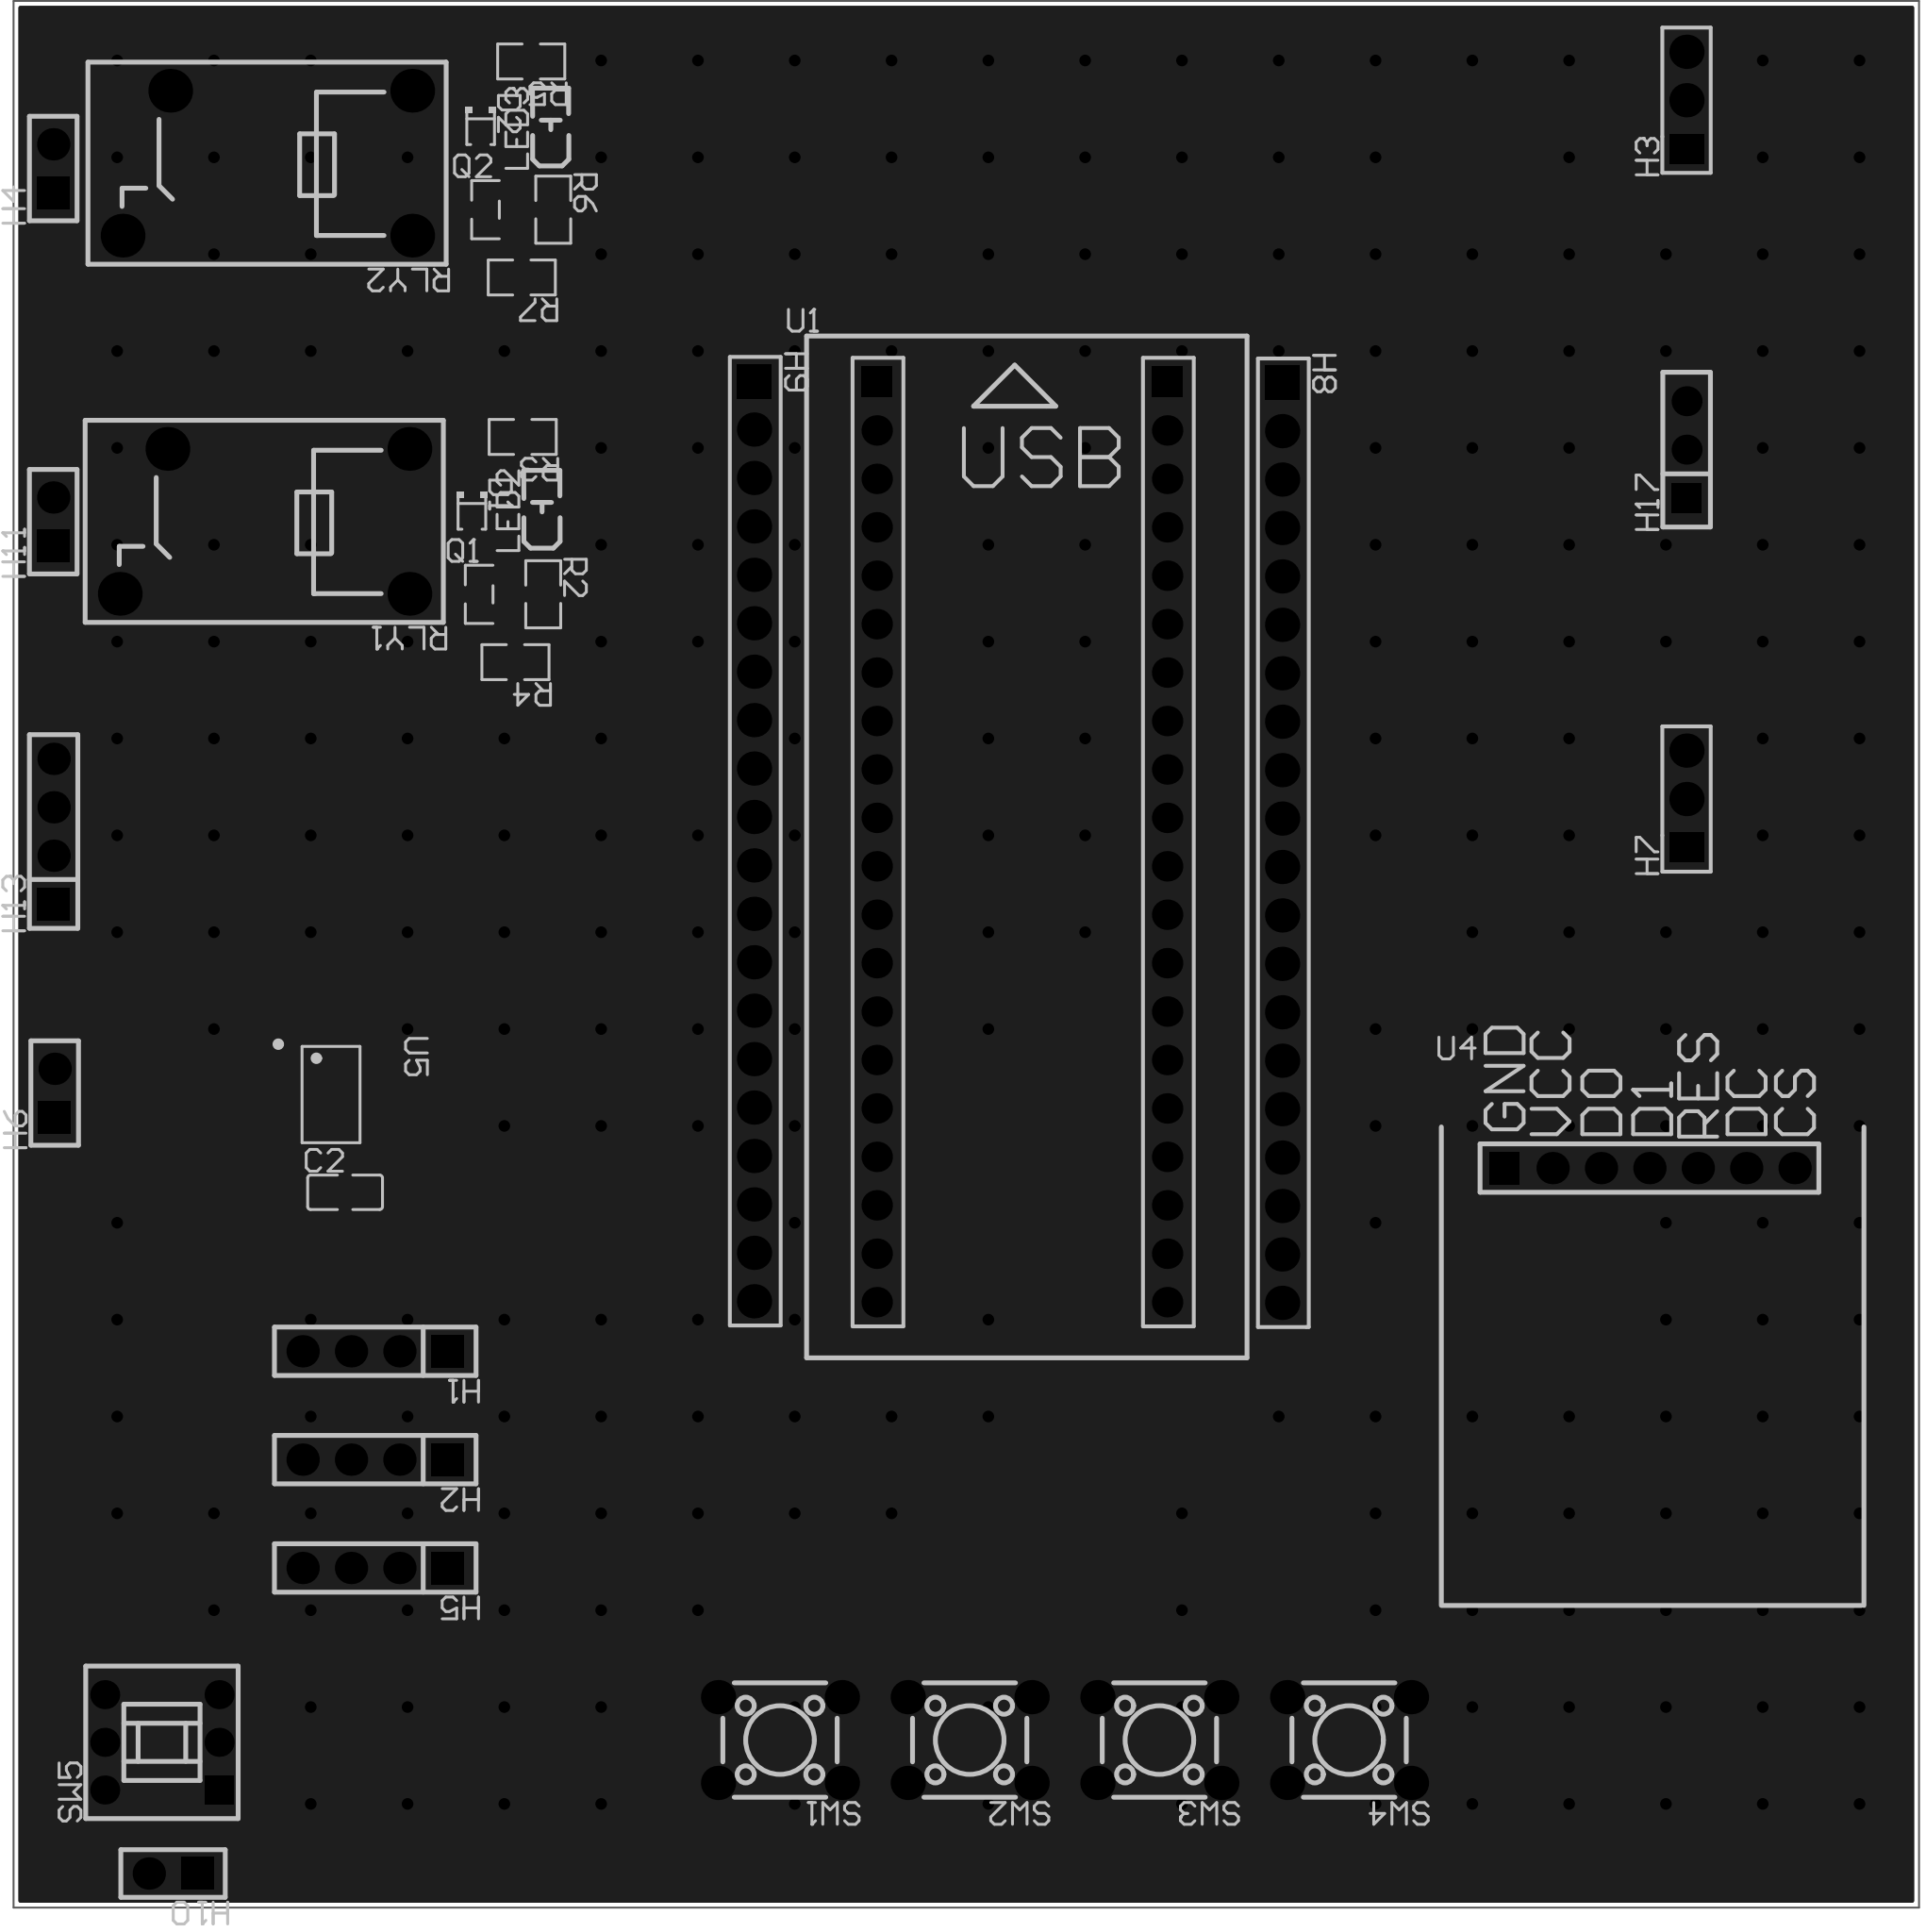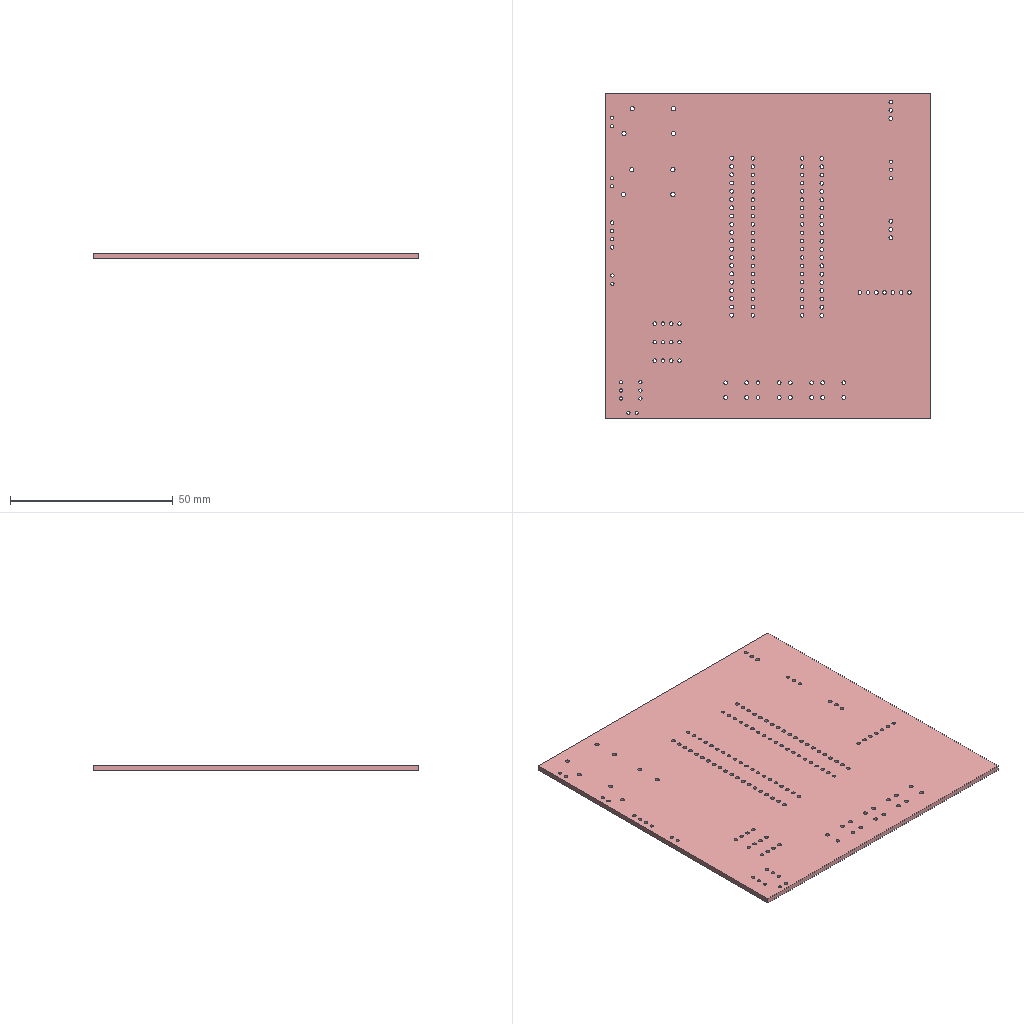Circuit board layout | Altium Designer | box 100 x 100 x 1.6 mm
Layer stack:
# Altium Designer layer stack of  (unit mm; dielectric type: 0 none, 1 core, 2 prepreg, 3 surface material)
index,name,kind,layer,copper_thickness_mm,dielectric_type,dielectric_thickness_mm,dielectric_material,dielectric_constant
0,Top Paste Mask Layer,other,,,,,,
1,Top Silkscreen Layer,other,,,,,,
2,Top Solder Mask Layer,dielectric,,,3,0.01,,3.3
3,Top Layer,copper,Top Layer,0.035,,,,
4,Dielectric1,dielectric,,,3,1.51,FR4,4.5
5,Bottom Layer,copper,Bottom Layer,0.035,,,,
6,Bottom Solder Mask Layer,dielectric,,,3,0.01,,3.3
7,Bottom Silkscreen Layer,other,,,,,,
8,Bottom Paste Mask Layer,other,,,,,,
# drill layer pairs: low layer,high layer
drill_pair,Top Layer,Bottom Layer
Part placement:
Designator,Comment,Layer,Footprint,Center-X(mm),Center-Y(mm),Rotation
C2,1uf,TopLayer,C0805,99.822,119.126,0
D1,1N4007WS,TopLayer,SOD-323_L1.8-W1.3-LS2.5-RD,106.477,154.806,270
D2,1N4007WS,TopLayer,SOD-323_L1.8-W1.3-LS2.5-RD,106.937,174.981,270
H1,,TopLayer,HDR-TH_4P-P2.54-V-F,101.405,110.788,180
H2,,TopLayer,HDR-TH_4P-P2.54-V-F,101.405,105.105,180
H3,Header-Male-2.54_1x3,TopLayer,HDR-TH_3P-P2.54-V-M-1,170.22,176.403,90
H4,,TopLayer,HDR-TH_2P-P2.54-V-F,84.506,172.821,90
H5,,TopLayer,HDR-TH_4P-P2.54-V-F,101.405,99.423,180
H6,,TopLayer,HDR-TH_2P-P2.54-V-F,84.582,124.333,90
H7,Header-Male-2.54_1x3,TopLayer,HDR-TH_3P-P2.54-V-M-1,170.22,139.752,90
H8,,TopLayer,HDR-TH_20P-P2.54-V-M-1,148.999,137.458,270
H9,,TopLayer,HDR-TH_20P-P2.54-V-M-1,121.285,137.541,270
H10,,TopLayer,HDR-TH_2P-P2.54-V-F,90.793,83.398,180
H11,,TopLayer,HDR-TH_2P-P2.54-V-F,84.506,154.298,90
H13,Header-Male-2.54_1x4,TopLayer,HDR-TH_4P-P2.54-V-M,84.526,138.049,90
H17,,TopLayer,HDR-TH_3P-P2.54-V-F,170.226,158.077,90
LED2,,TopLayer,LED_0805,110.155,155.01,90
LED3,,TopLayer,LED_0805,110.615,175.057,90
Q1,SS8050_C2150,TopLayer,SOT-23-3_L2.9-W1.3-P1.90-LS2.4-BR,106.858,150.488,0
Q2,SS8050_C2150,TopLayer,SOT-23-3_L2.9-W1.3-P1.90-LS2.4-BR,107.191,170.662,0
R2,4.7kΩ,TopLayer,R0805,110.221,150.49,270
R3,4.7kΩ,TopLayer,R0805,109.144,158.743,180
R4,10k,TopLayer,R0805,108.763,146.932,180
R5,4.7kΩ,TopLayer,R0805,109.591,178.435,180
R6,4.7kΩ,TopLayer,R0805,110.747,170.662,270
R7,10k,TopLayer,R0805,109.096,167.107,180
RLY1,JZC-32F/005-HS3(555),TopLayer,RELAY-TH_JZC-32F-XXXHXX,95.6,154.316,180
RLY2,JZC-32F/005-HS3(555),TopLayer,RELAY-TH_JZC-32F-XXXHXX,95.748,173.101,180
SW1,TS665CJ,TopLayer,SW-TH_4P-L6.0-W6.0-P4.50-LS6.5,122.647,90.398,180
SW2,TS665CJ,TopLayer,SW-TH_4P-L6.0-W6.0-P4.50-LS6.5,132.602,90.398,180
SW3,TS665CJ,TopLayer,SW-TH_4P-L6.0-W6.0-P4.50-LS6.5,142.558,90.398,180
SW4,TS665CJ,TopLayer,SW-TH_4P-L6.0-W6.0-P4.50-LS6.5,152.513,90.398,180
SW5,XKB8080-Z,TopLayer,SW-TH_6P-L8.0-W8.0-P2.50,90.21,90.278,90
U1,,TopLayer,STM32最小系统,135.345,137.494,0
U4,,TopLayer,OLED12864/7针,168.275,120.396,0
U5,L9110S_C2895059,TopLayer,SOP-8_L5.0-W4.0-P1.27-LS6.0-BL,99.085,124.251,270
Pad and via stacks:
# Altium Designer via and pad stacks of  (unit mm). Each distinct definition once, with the count of objects using it.
# via: kind,start_layer,end_layer,hole_mm,diameter_mm,mode(0 simple;1 top-mid-bottom;2 full stack),diameter_per_layer,count,example_net
# pad: kind,layer,hole_mm,hole_type(0 round;1 square;2 slot),plating,top_size,top_shape(1 round;2 rect;3 octagon;9 rounded rect),mid_size,bottom_size,mode,footprint,size_per_layer,count,example
pad,Top Layer,0,0,plated,1.41x1.35,2,1.41x1.35,1.41x1.35,0,C0805,,2,C2.2
pad,Top Layer,0,0,plated,1x0.75,2,1x0.75,1x0.75,0,SOD-323_L1.8-W1.3-LS2.5-RD,,4,D1.2
pad,Top Layer,0,0,plated,1x1.25,2,1x1.25,1x1.25,0,LED_0805,,4,LED2.2
pad,Top Layer,0,0,plated,1.25x0.7,2,1.25x0.7,1.25x0.7,0,SOT-23-3_L2.9-W1.3-P1.90-LS2.4-BR,,6,Q1.1
pad,Top Layer,0,0,plated,1.133x1.377,2,1.133x1.377,1.133x1.377,0,R0805,,12,R2.2
pad,Top Layer,0,0,plated,0.574x2.035,1,0.574x2.035,0.574x2.035,0,SOP-8_L5.0-W4.0-P1.27-LS6.0-BL,,8,U5.1
pad,Multi-Layer,1.1,0,plated,1.7x1.7,2,1.7x1.7,1.7x1.7,0,HDR-TH_4P-P2.54-V-F,,3,H1.1
pad,Multi-Layer,1.1,0,plated,1.7x1.7,1,1.7x1.7,1.7x1.7,0,HDR-TH_4P-P2.54-V-F,,9,H1.2
pad,Multi-Layer,1.2,0,plated,1.8x1.8,1,1.8x1.8,1.8x1.8,0,HDR-TH_3P-P2.54-V-M-1,,4,H3.3
pad,Multi-Layer,1.2,0,plated,1.575x1.8,2,1.575x1.8,1.575x1.8,0,HDR-TH_3P-P2.54-V-M-1,,2,H3.1
pad,Multi-Layer,1,0,plated,1.7x1.7,2,1.7x1.7,1.7x1.7,0,HDR-TH_2P-P2.54-V-F,,4,H4.1
pad,Multi-Layer,1,0,plated,1.7x1.7,1,1.7x1.7,1.7x1.7,0,HDR-TH_2P-P2.54-V-F,,4,H4.2
pad,Multi-Layer,1.2,0,plated,1.8x1.8,1,1.8x1.8,1.8x1.8,0,HDR-TH_20P-P2.54-V-M-1,,38,H8.20
pad,Multi-Layer,1.2,0,plated,1.8x1.8,2,1.8x1.8,1.8x1.8,0,HDR-TH_20P-P2.54-V-M-1,,2,H8.1
pad,Multi-Layer,1.1,0,plated,1.7x1.7,2,1.7x1.7,1.7x1.7,0,HDR-TH_4P-P2.54-V-M,,1,H13.1
pad,Multi-Layer,1.1,0,plated,1.7x1.7,1,1.7x1.7,1.7x1.7,0,HDR-TH_4P-P2.54-V-M,,3,H13.2
pad,Multi-Layer,1.02,0,plated,1.575x1.575,1,1.575x1.575,1.575x1.575,0,HDR-TH_3P-P2.54-V-F,,2,H17.3
pad,Multi-Layer,1.02,0,plated,1.575x1.575,2,1.575x1.575,1.575x1.575,0,HDR-TH_3P-P2.54-V-F,,1,H17.1
pad,Multi-Layer,1.3,0,plated,2.3x2.3,1,2.3x2.3,2.3x2.3,0,RELAY-TH_JZC-32F-XXXHXX,,8,RLY1.1
pad,Multi-Layer,1.2,0,plated,1.8x1.8,1,1.8x1.8,1.8x1.8,0,SW-TH_4P-L6.0-W6.0-P4.50-LS6.5,,16,SW1.1
pad,Multi-Layer,1,0,plated,1.524x1.524,1,1.524x1.524,1.524x1.524,0,SW-TH_6P-L8.0-W8.0-P2.50,,5,SW5.3
pad,Multi-Layer,1,0,plated,1.524x1.524,2,1.524x1.524,1.524x1.524,0,SW-TH_6P-L8.0-W8.0-P2.50,,1,SW5.1
pad,Multi-Layer,1.05,0,plated,1.6x1.6,1,1.6x1.6,1.6x1.6,0,STM32\u00D7\u00EE\u00D0\u00A1\u00CF\u00B5\u00CD\u00B3,,38,U1.20
pad,Multi-Layer,1.05,0,plated,1.6x1.6,2,1.6x1.6,1.6x1.6,0,STM32\u00D7\u00EE\u00D0\u00A1\u00CF\u00B5\u00CD\u00B3,,2,U1.1
pad,Multi-Layer,1.1,0,plated,1.7x1.7,1,1.7x1.7,1.7x1.7,0,OLED12864/7\u00D5\u00EB,,6,U4.7
pad,Multi-Layer,1.1,0,plated,1.575x1.7,2,1.575x1.7,1.575x1.7,0,OLED12864/7\u00D5\u00EB,,1,U4.1
via,Top Layer,Bottom Layer,0.3048,0.61,0,,262,GND
Copper pours:
name,layer,net,type(0 solid;1 hatched;2 none)
Top Layer-GND,Top Layer,GND,0
Bottom Layer-GND,Bottom Layer,GND,0